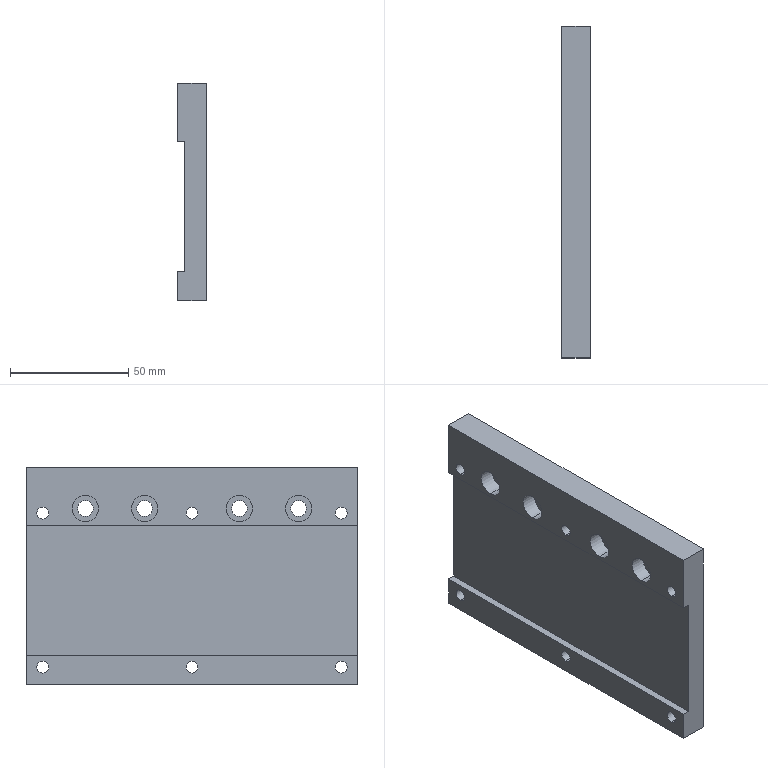Part | STEP file | LM-05-1163 modified_default | 1 solid | 42 faces | box 12 x 140 x 92 mm | volume 126847 mm3 | cylinder 28 | plane 14 | commonest cylinder face diameters 5 x12 6.6 x8 11 x8